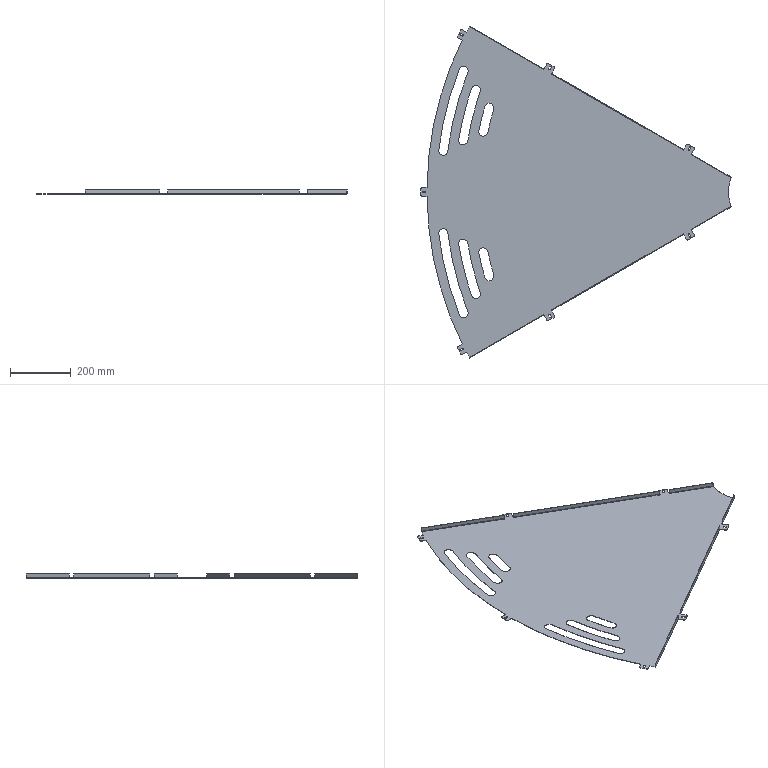Part | SolidWorks | features SMBaseFlange 8, EdgeFlange 6, ICE 2, BreakCorner 1, FlatPattern 1, SheetMetal 1 | 1 solid | 183 faces | box 1022 x 1094 x 15 mm | volume 731412 mm3 | plane 94 | cylinder 87 | spline 2 | commonest cylinder face diameters 6 x21 10 x15 1.473 x6 3.873 x6 30.001 x4 30.003 x4